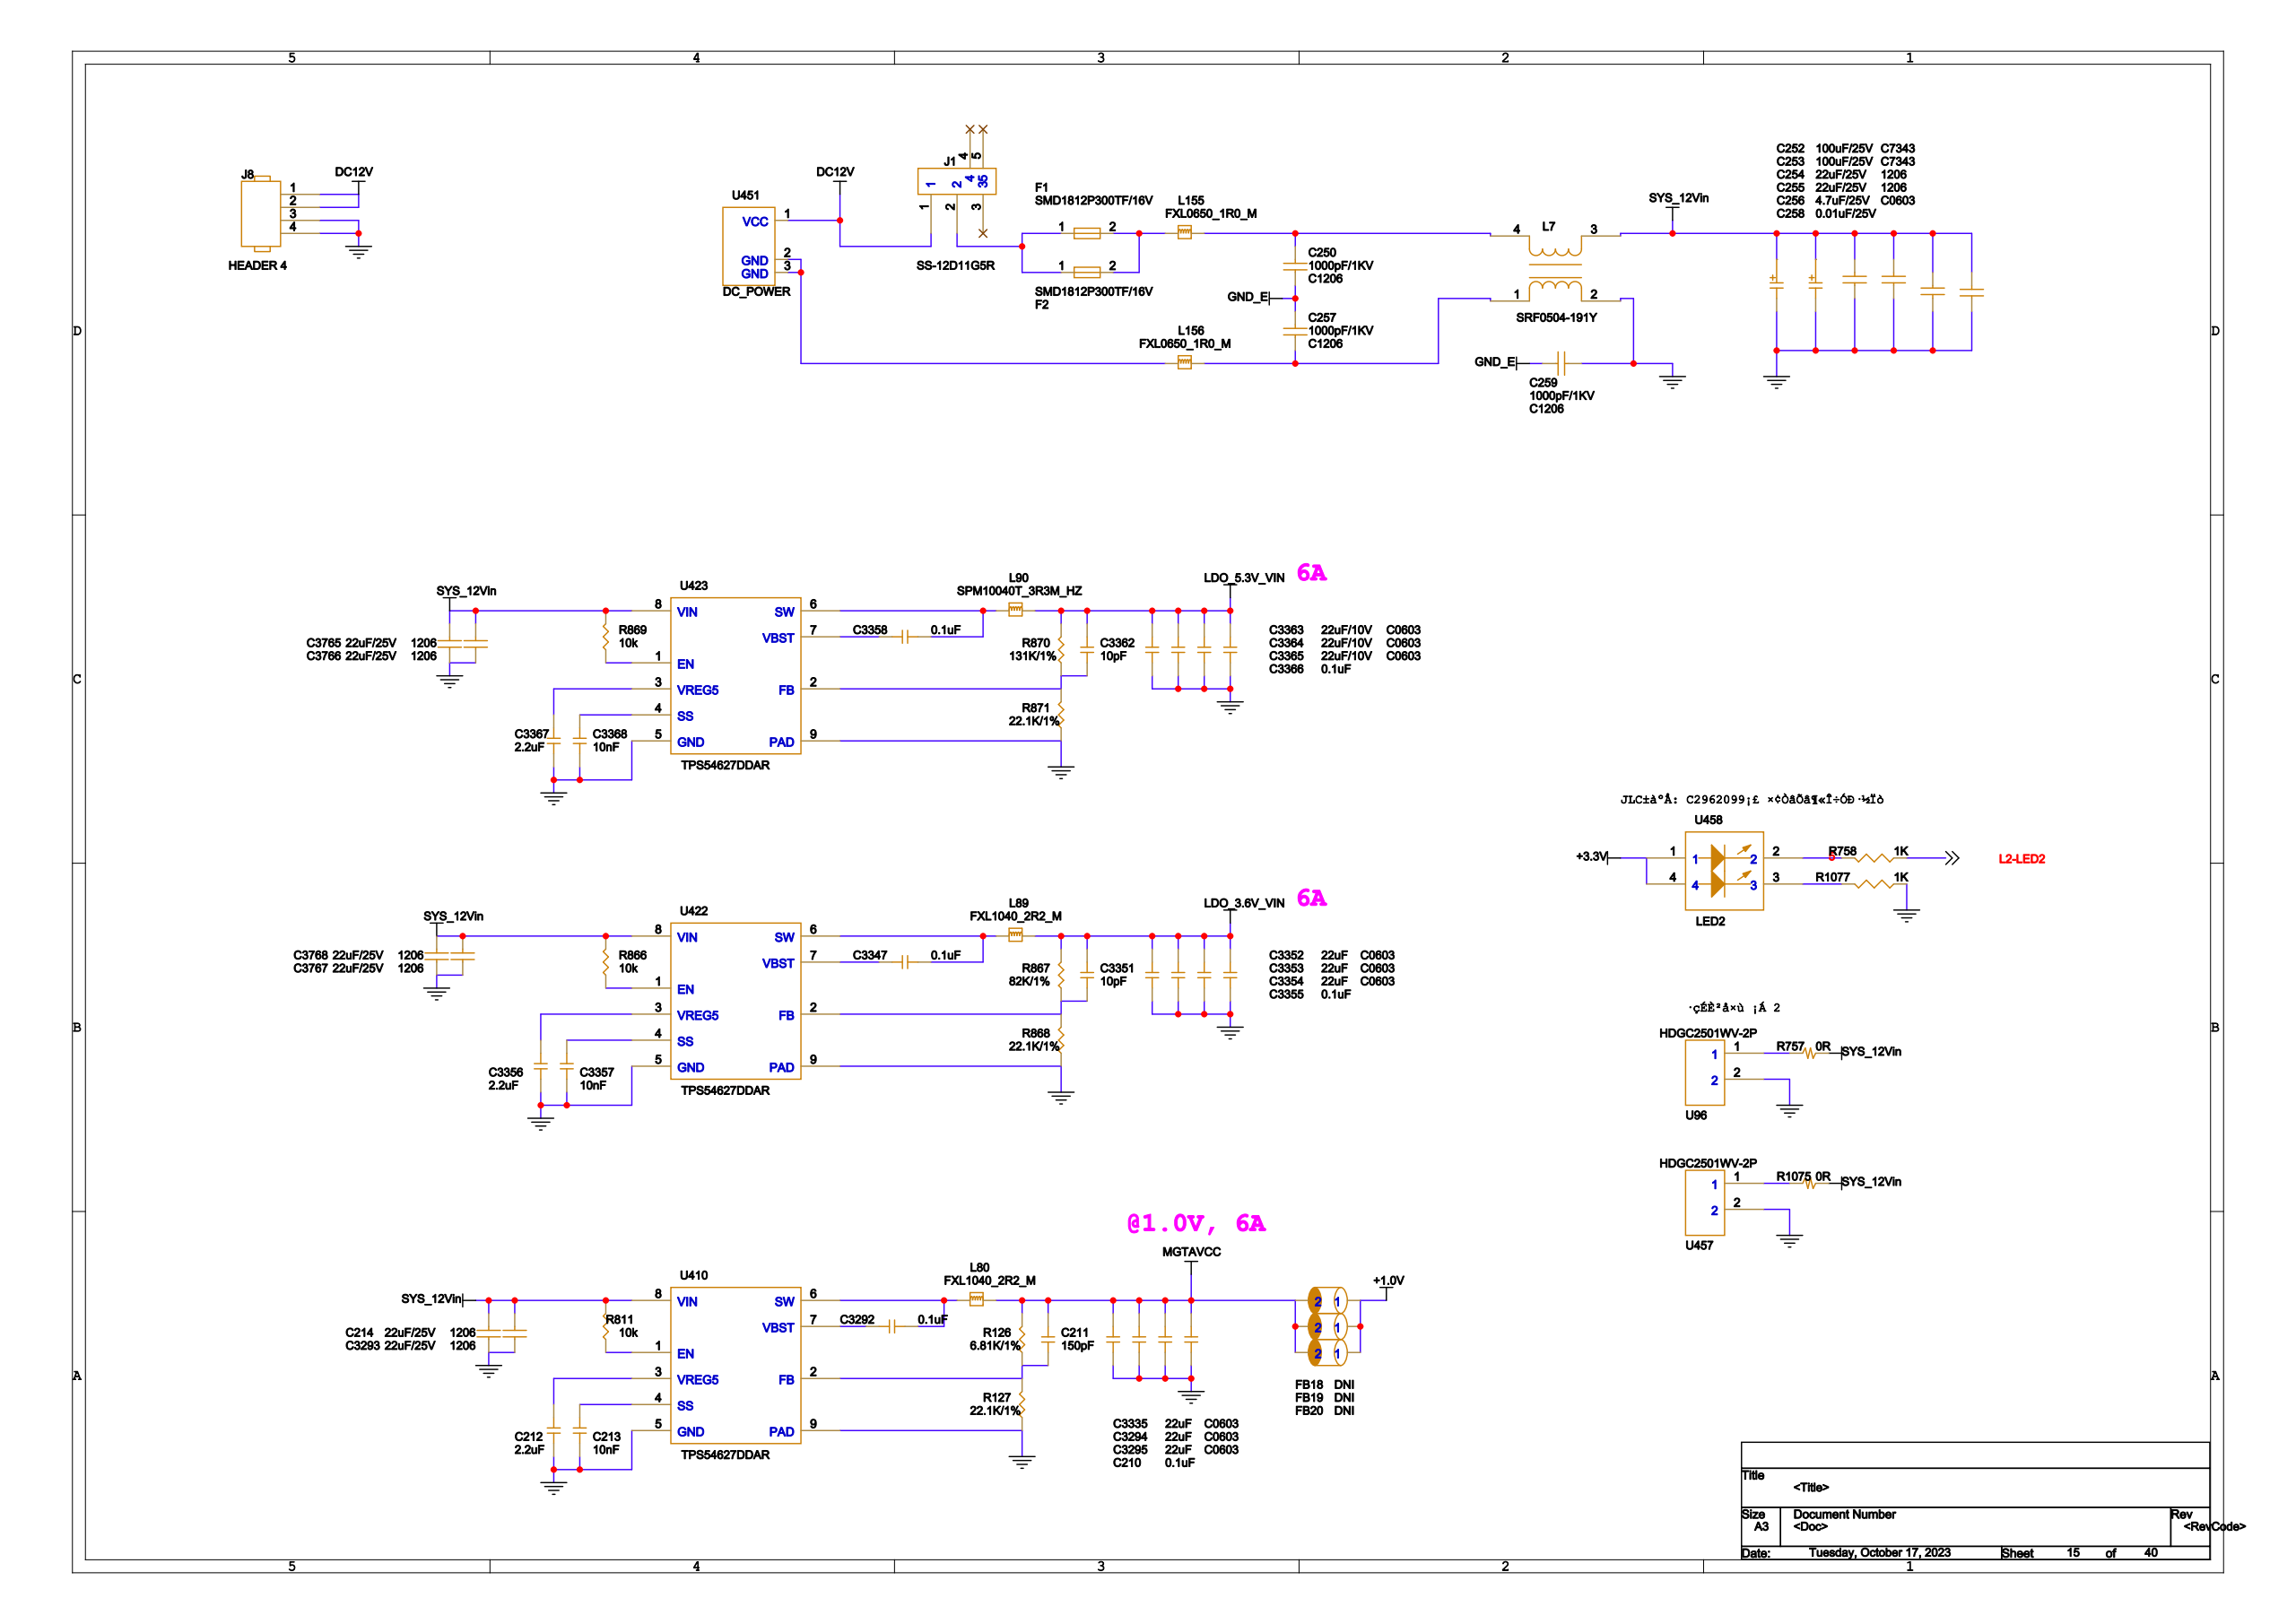Circuit board | Cadence Allegro | 1793 parts | 1223 nets | one sheet of the schematic
Parts on this sheet (reference | value | footprint):
C210 | 0.1uF | C0402
C211 | 150pF | C0402
C212 | 2.2uF | C0402
C213 | 10nF | C0402
C214 | 22uF/25V | 1206
C250 | 1000pF/1KV | C1206
C252 | 100uF/25V | C7343
C253 | 100uF/25V | C7343
C254 | 22uF/25V | 1206
C255 | 22uF/25V | 1206
C256 | 4.7uF/25V | C0603
C257 | 1000pF/1KV | C1206
C258 | 0.01uF/25V | C0402
C259 | 1000pF/1KV | C1206
C3292 | 0.1uF | C0402
C3293 | 22uF/25V | 1206
C3294 | 22uF | C0603
C3295 | 22uF | C0603
C3335 | 22uF | C0603
C3347 | 0.1uF | C0402
C3351 | 10pF | C0402
C3352 | 22uF | C0603
C3353 | 22uF | C0603
C3354 | 22uF | C0603
C3355 | 0.1uF | C0402
C3356 | 2.2uF | C0402
C3357 | 10nF | C0402
C3358 | 0.1uF | C0402
C3362 | 10pF | C0402
C3363 | 22uF/10V | C0603
C3364 | 22uF/10V | C0603
C3365 | 22uF/10V | C0603
C3366 | 0.1uF | C0402
C3367 | 2.2uF | C0402
C3368 | 10nF | C0402
C3765 | 22uF/25V | 1206
C3766 | 22uF/25V | 1206
C3767 | 22uF/25V | 1206
C3768 | 22uF/25V | 1206
F1 | SMD1812P300TF/16V | F1812
F2 | SMD1812P300TF/16V | F1812
FB18 | DNI | FB0603
FB19 | DNI | FB0603
FB20 | DNI | FB0603
J1 | SS-12D11G5R | SW-TH_SS-12D11G5R
J8 | HEADER 4 | CH_508_1X4P
L7 | SRF0504-191Y | SRF0504-191Y
L80 | FXL1040_2R2_M | SMD_11_5X10
L89 | FXL1040_2R2_M | SMD_11_5X10
L90 | SPM10040T_3R3M_HZ | SMD_10X10MM
L155 | FXL0650_1R0_M | SMD_SMD_7X6_6
L156 | FXL0650_1R0_M | SMD_SMD_7X6_6
R126 | 6.81K/1% | R0402
R127 | 22.1K/1% | R0402
R757 | 0R | R0402
R758 | 1K | R0402
R811 | 10k | R0402
R866 | 10k | R0402
R867 | 82K/1% | R0402
R868 | 22.1K/1% | R0402
R869 | 10k | R0402
R870 | 131K/1% | R0402
R871 | 22.1K/1% | R0402
R1075 | 0R | R0402
R1077 | 1K | R0402
U96 | HDGC2501WV-2P | CONN-TH_XH2_5-2P
U410 | TPS54627DDAR | POWER-SO8
U422 | TPS54627DDAR | POWER-SO8
U423 | TPS54627DDAR | POWER-SO8
U451 | DC_POWER | DC-IN-TH_DC-005-5A-2_0
U457 | HDGC2501WV-2P | CONN-TH_XH2_5-2P
U458 | LED2 | LED-TH_4P-L11_8-W4_3-P2_54
Nets of these parts (net: part-pin ...):
GND: C210-1 C212-1 C213-1 C214-1 C252-2 C253-2 C254-1 C255-1 C256-2 C258-1 C259-2 C3293-1 C3294-1 C3295-1 C3335-1 C3352-1 C3353-1 C3354-1 C3355-1 C3356-1 C3357-1 C3363-1 C3364-1 C3365-1 C3366-1 C3367-1 C3368-1 C3765-1 C3766-1 C3767-1 C3768-1 J8-3 J8-4 L7-2 R127-2 R868-2 R871-2 R1077-2 U96-2 U410-5 U410-9 U422-5 U422-9 U423-5 U423-9 U457-2
+3.3V: U458-1 U458-4
LDO_5.3V_VIN: C3362-2 C3363-2 C3364-2 C3365-2 C3366-2 L90-2 R870-1
SYS_12VIN: C214-2 C252-1 C253-1 C254-2 C255-2 C256-1 C258-2 C3293-2 C3765-2 C3766-2 C3767-2 C3768-2 L7-3 R757-1 R811-1 R866-1 R869-1 R1075-1 U410-8 U422-8 U423-8
N18646943: R811-2 U410-1
LDO_3.6V_VIN: C3351-2 C3352-2 C3353-2 C3354-2 C3355-2 L89-2 R867-1
N16933439: R866-2 U422-1
N16934712: R869-2 U423-1
+1.0V: FB18-1 FB19-1 FB20-1
DC12V: J1-1 J8-1 J8-2 U451-1
N16585129: F1-1 F2-1 J1-2
N16585261: L156-1 U451-2 U451-3
N18453707: R758-1 U458-2
N18453706: R1077-1 U458-3
MGTAVCC: C210-2 C211-2 C3294-2 C3295-2 C3335-2 FB18-2 FB19-2 FB20-2 L80-2 R126-1
N18646987: C213-2 U410-4
N16933507: C3357-2 U422-4
N16934780: C3368-2 U423-4
N18646959: C212-2 U410-3
N16933459: C3356-2 U422-3
N16934732: C3367-2 U423-3
N18646760: C3292-2 L80-1 U410-6
N16933273: C3347-2 L89-1 U422-6
N16585137: F1-2 F2-2 L155-1
N16585149: C250-2 L7-4 L155-2
N16585337: C257-1 L7-1 L156-2
N16934546: C3358-2 L90-1 U423-6
N18344542: R1075-2 U457-1
N16588210: R757-2 U96-1
N18646947: C211-1 R126-2 R127-1 U410-2
N18646848: C3292-1 U410-7
N16933447: C3351-1 R867-2 R868-1 U422-2
N16933363: C3347-1 U422-7
N16934720: C3362-1 R870-2 R871-1 U423-2
N16934636: C3358-1 U423-7
GND_E: C250-1 C257-2 C259-1
L2-LED2: R758-2